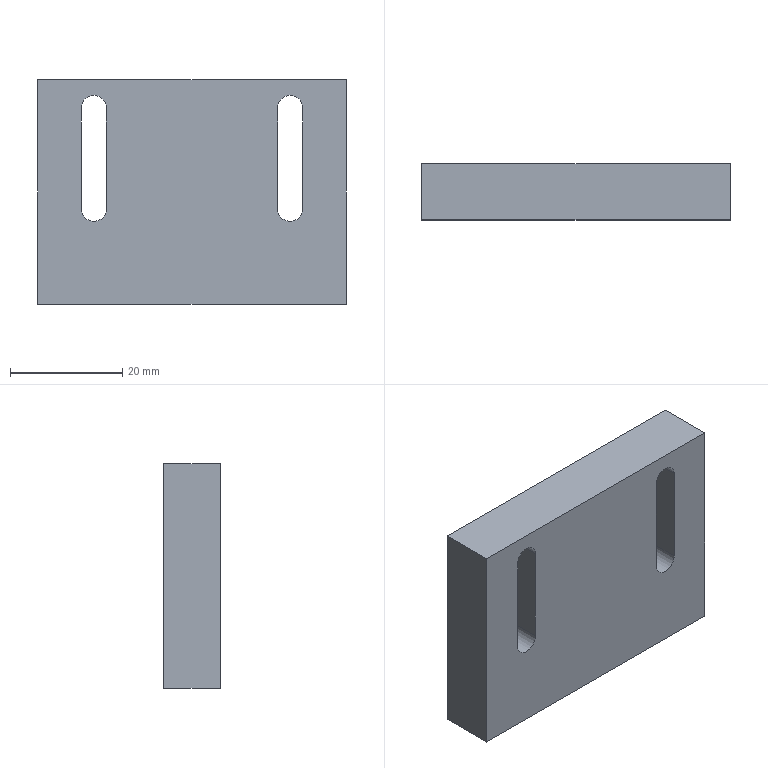Part | STEP file | PN_0007 fixture positioning -V-shape edge 1-2_Default | 1 solid | 16 faces | box 55 x 10 x 40 mm | volume 20062 mm3 | plane 10 | cylinder 6 | commonest cylinder face diameters 4.5 x6
STEP:
#1=CARTESIAN_POINT('',(0.,0.,0.));
#2=DIRECTION('',(0.,0.,1.));
#3=DIRECTION('',(1.,0.,0.));
#4=AXIS2_PLACEMENT_3D('',#1,#2,#3);
#5=CARTESIAN_POINT('',(19.75,0.,15.));
#6=VERTEX_POINT('',#5);
#7=CARTESIAN_POINT('',(19.75,10.,15.));
#8=VERTEX_POINT('',#7);
#9=CARTESIAN_POINT('',(19.75,-2.5,15.));
#10=DIRECTION('',(0.,1.,0.));
#11=VECTOR('',#10,1.);
#12=LINE('',#9,#11);
#13=CARTESIAN_POINT('',(17.5,-2.5,15.));
#14=DIRECTION('',(0.,1.,0.));
#15=DIRECTION('',(0.,0.,1.));
#16=AXIS2_PLACEMENT_3D('',#13,#14,#15);
#17=CYLINDRICAL_SURFACE('',#16,2.25);
#18=CARTESIAN_POINT('',(1.571,0.));
#19=DIRECTION('',(0.,1.));
#20=VECTOR('',#19,1.);
#21=LINE('',#18,#20);
#22=(GEOMETRIC_REPRESENTATION_CONTEXT(2)PARAMETRIC_REPRESENTATION_CONTEXT()REPRESENTATION_CONTEXT('',''));
#23=DEFINITIONAL_REPRESENTATION('',(#21),#22);
#24=PCURVE('',#17,#23);
#25=CARTESIAN_POINT('',(19.75,-2.5,-3.));
#26=DIRECTION('',(1.,0.,0.));
#27=DIRECTION('',(0.,0.,-1.));
#28=AXIS2_PLACEMENT_3D('',#25,#26,#27);
#29=PLANE('',#28);
#30=CARTESIAN_POINT('',(-18.,0.));
#31=DIRECTION('',(0.,1.));
#32=VECTOR('',#31,1.);
#33=LINE('',#30,#32);
#34=(GEOMETRIC_REPRESENTATION_CONTEXT(2)PARAMETRIC_REPRESENTATION_CONTEXT()REPRESENTATION_CONTEXT('',''));
#35=DEFINITIONAL_REPRESENTATION('',(#33),#34);
#36=PCURVE('',#29,#35);
#37=SURFACE_CURVE('',#12,(#24,#36),.PCURVE_S1.);
#38=EDGE_CURVE('',#6,#8,#37,.T.);
#39=ORIENTED_EDGE('',*,*,#38,.T.);
#40=CARTESIAN_POINT('',(17.5,10.,17.25));
#41=VERTEX_POINT('',#40);
#42=CARTESIAN_POINT('',(17.5,10.,15.));
#43=DIRECTION('',(0.,1.,0.));
#44=DIRECTION('',(0.,0.,1.));
#45=AXIS2_PLACEMENT_3D('',#42,#43,#44);
#46=CIRCLE('',#45,2.25);
#47=CARTESIAN_POINT('',(0.,12.5));
#48=DIRECTION('',(1.,0.));
#49=VECTOR('',#48,1.);
#50=LINE('',#47,#49);
#51=(GEOMETRIC_REPRESENTATION_CONTEXT(2)PARAMETRIC_REPRESENTATION_CONTEXT()REPRESENTATION_CONTEXT('',''));
#52=DEFINITIONAL_REPRESENTATION('',(#50),#51);
#53=PCURVE('',#17,#52);
#54=CARTESIAN_POINT('',(0.,10.,0.));
#55=DIRECTION('',(0.,1.,0.));
#56=DIRECTION('',(0.,0.,1.));
#57=AXIS2_PLACEMENT_3D('',#54,#55,#56);
#58=PLANE('',#57);
#59=CARTESIAN_POINT('',(15.,17.5));
#60=DIRECTION('',(1.,0.));
#61=AXIS2_PLACEMENT_2D('',#59,#60);
#62=CIRCLE('',#61,2.25);
#63=(GEOMETRIC_REPRESENTATION_CONTEXT(2)PARAMETRIC_REPRESENTATION_CONTEXT()REPRESENTATION_CONTEXT('',''));
#64=DEFINITIONAL_REPRESENTATION('',(#62),#63);
#65=PCURVE('',#58,#64);
#66=SURFACE_CURVE('',#46,(#53,#65),.PCURVE_S1.);
#67=EDGE_CURVE('',#41,#8,#66,.T.);
#68=ORIENTED_EDGE('',*,*,#67,.F.);
#69=CARTESIAN_POINT('',(17.5,0.,17.25));
#70=VERTEX_POINT('',#69);
#71=CARTESIAN_POINT('',(17.5,-2.5,17.25));
#72=DIRECTION('',(0.,1.,0.));
#73=VECTOR('',#72,1.);
#74=LINE('',#71,#73);
#75=CARTESIAN_POINT('',(0.,0.));
#76=DIRECTION('',(0.,1.));
#77=VECTOR('',#76,1.);
#78=LINE('',#75,#77);
#79=(GEOMETRIC_REPRESENTATION_CONTEXT(2)PARAMETRIC_REPRESENTATION_CONTEXT()REPRESENTATION_CONTEXT('',''));
#80=DEFINITIONAL_REPRESENTATION('',(#78),#79);
#81=PCURVE('',#17,#80);
#82=CARTESIAN_POINT('',(17.5,-2.5,15.));
#83=DIRECTION('',(0.,1.,0.));
#84=DIRECTION('',(0.,0.,1.));
#85=AXIS2_PLACEMENT_3D('',#82,#83,#84);
#86=CYLINDRICAL_SURFACE('',#85,2.25);
#87=CARTESIAN_POINT('',(6.283,0.));
#88=DIRECTION('',(0.,1.));
#89=VECTOR('',#88,1.);
#90=LINE('',#87,#89);
#91=(GEOMETRIC_REPRESENTATION_CONTEXT(2)PARAMETRIC_REPRESENTATION_CONTEXT()REPRESENTATION_CONTEXT('',''));
#92=DEFINITIONAL_REPRESENTATION('',(#90),#91);
#93=PCURVE('',#86,#92);
#94=SURFACE_CURVE('',#74,(#81,#93),.PCURVE_S1.);
#95=EDGE_CURVE('',#70,#41,#94,.T.);
#96=ORIENTED_EDGE('',*,*,#95,.F.);
#97=CARTESIAN_POINT('',(17.5,0.,15.));
#98=DIRECTION('',(0.,1.,0.));
#99=DIRECTION('',(0.,0.,1.));
#100=AXIS2_PLACEMENT_3D('',#97,#98,#99);
#101=CIRCLE('',#100,2.25);
#102=CARTESIAN_POINT('',(0.,2.5));
#103=DIRECTION('',(1.,0.));
#104=VECTOR('',#103,1.);
#105=LINE('',#102,#104);
#106=(GEOMETRIC_REPRESENTATION_CONTEXT(2)PARAMETRIC_REPRESENTATION_CONTEXT()REPRESENTATION_CONTEXT('',''));
#107=DEFINITIONAL_REPRESENTATION('',(#105),#106);
#108=PCURVE('',#17,#107);
#109=CARTESIAN_POINT('',(0.,0.,0.));
#110=DIRECTION('',(0.,1.,0.));
#111=DIRECTION('',(0.,0.,1.));
#112=AXIS2_PLACEMENT_3D('',#109,#110,#111);
#113=PLANE('',#112);
#114=CARTESIAN_POINT('',(15.,17.5));
#115=DIRECTION('',(1.,0.));
#116=AXIS2_PLACEMENT_2D('',#114,#115);
#117=CIRCLE('',#116,2.25);
#118=(GEOMETRIC_REPRESENTATION_CONTEXT(2)PARAMETRIC_REPRESENTATION_CONTEXT()REPRESENTATION_CONTEXT('',''));
#119=DEFINITIONAL_REPRESENTATION('',(#117),#118);
#120=PCURVE('',#113,#119);
#121=SURFACE_CURVE('',#101,(#108,#120),.PCURVE_S1.);
#122=EDGE_CURVE('',#70,#6,#121,.T.);
#123=ORIENTED_EDGE('',*,*,#122,.T.);
#124=EDGE_LOOP('',(#39,#68,#96,#123));
#125=FACE_BOUND('',#124,.F.);
#126=ADVANCED_FACE('',(#125),#17,.F.);
#127=CARTESIAN_POINT('',(-15.25,0.,15.));
#128=VERTEX_POINT('',#127);
#129=CARTESIAN_POINT('',(-15.25,10.,15.));
#130=VERTEX_POINT('',#129);
#131=CARTESIAN_POINT('',(-15.25,-2.5,15.));
#132=DIRECTION('',(0.,1.,0.));
#133=VECTOR('',#132,1.);
#134=LINE('',#131,#133);
#135=CARTESIAN_POINT('',(-17.5,-2.5,15.));
#136=DIRECTION('',(0.,1.,0.));
#137=DIRECTION('',(0.,0.,1.));
#138=AXIS2_PLACEMENT_3D('',#135,#136,#137);
#139=CYLINDRICAL_SURFACE('',#138,2.25);
#140=CARTESIAN_POINT('',(1.571,0.));
#141=DIRECTION('',(0.,1.));
#142=VECTOR('',#141,1.);
#143=LINE('',#140,#142);
#144=(GEOMETRIC_REPRESENTATION_CONTEXT(2)PARAMETRIC_REPRESENTATION_CONTEXT()REPRESENTATION_CONTEXT('',''));
#145=DEFINITIONAL_REPRESENTATION('',(#143),#144);
#146=PCURVE('',#139,#145);
#147=CARTESIAN_POINT('',(-15.25,-2.5,-3.));
#148=DIRECTION('',(1.,0.,0.));
#149=DIRECTION('',(0.,0.,-1.));
#150=AXIS2_PLACEMENT_3D('',#147,#148,#149);
#151=PLANE('',#150);
#152=CARTESIAN_POINT('',(-18.,0.));
#153=DIRECTION('',(0.,1.));
#154=VECTOR('',#153,1.);
#155=LINE('',#152,#154);
#156=(GEOMETRIC_REPRESENTATION_CONTEXT(2)PARAMETRIC_REPRESENTATION_CONTEXT()REPRESENTATION_CONTEXT('',''));
#157=DEFINITIONAL_REPRESENTATION('',(#155),#156);
#158=PCURVE('',#151,#157);
#159=SURFACE_CURVE('',#134,(#146,#158),.PCURVE_S1.);
#160=EDGE_CURVE('',#128,#130,#159,.T.);
#161=ORIENTED_EDGE('',*,*,#160,.T.);
#162=CARTESIAN_POINT('',(-17.5,10.,17.25));
#163=VERTEX_POINT('',#162);
#164=CARTESIAN_POINT('',(-17.5,10.,15.));
#165=DIRECTION('',(0.,1.,0.));
#166=DIRECTION('',(0.,0.,1.));
#167=AXIS2_PLACEMENT_3D('',#164,#165,#166);
#168=CIRCLE('',#167,2.25);
#169=CARTESIAN_POINT('',(0.,12.5));
#170=DIRECTION('',(1.,0.));
#171=VECTOR('',#170,1.);
#172=LINE('',#169,#171);
#173=(GEOMETRIC_REPRESENTATION_CONTEXT(2)PARAMETRIC_REPRESENTATION_CONTEXT()REPRESENTATION_CONTEXT('',''));
#174=DEFINITIONAL_REPRESENTATION('',(#172),#173);
#175=PCURVE('',#139,#174);
#176=CARTESIAN_POINT('',(15.,-17.5));
#177=DIRECTION('',(1.,0.));
#178=AXIS2_PLACEMENT_2D('',#176,#177);
#179=CIRCLE('',#178,2.25);
#180=(GEOMETRIC_REPRESENTATION_CONTEXT(2)PARAMETRIC_REPRESENTATION_CONTEXT()REPRESENTATION_CONTEXT('',''));
#181=DEFINITIONAL_REPRESENTATION('',(#179),#180);
#182=PCURVE('',#58,#181);
#183=SURFACE_CURVE('',#168,(#175,#182),.PCURVE_S1.);
#184=EDGE_CURVE('',#163,#130,#183,.T.);
#185=ORIENTED_EDGE('',*,*,#184,.F.);
#186=CARTESIAN_POINT('',(-17.5,0.,17.25));
#187=VERTEX_POINT('',#186);
#188=CARTESIAN_POINT('',(-17.5,-2.5,17.25));
#189=DIRECTION('',(0.,1.,0.));
#190=VECTOR('',#189,1.);
#191=LINE('',#188,#190);
#192=CARTESIAN_POINT('',(0.,0.));
#193=DIRECTION('',(0.,1.));
#194=VECTOR('',#193,1.);
#195=LINE('',#192,#194);
#196=(GEOMETRIC_REPRESENTATION_CONTEXT(2)PARAMETRIC_REPRESENTATION_CONTEXT()REPRESENTATION_CONTEXT('',''));
#197=DEFINITIONAL_REPRESENTATION('',(#195),#196);
#198=PCURVE('',#139,#197);
#199=CARTESIAN_POINT('',(-17.5,-2.5,15.));
#200=DIRECTION('',(0.,1.,0.));
#201=DIRECTION('',(0.,0.,1.));
#202=AXIS2_PLACEMENT_3D('',#199,#200,#201);
#203=CYLINDRICAL_SURFACE('',#202,2.25);
#204=CARTESIAN_POINT('',(6.283,0.));
#205=DIRECTION('',(0.,1.));
#206=VECTOR('',#205,1.);
#207=LINE('',#204,#206);
#208=(GEOMETRIC_REPRESENTATION_CONTEXT(2)PARAMETRIC_REPRESENTATION_CONTEXT()REPRESENTATION_CONTEXT('',''));
#209=DEFINITIONAL_REPRESENTATION('',(#207),#208);
#210=PCURVE('',#203,#209);
#211=SURFACE_CURVE('',#191,(#198,#210),.PCURVE_S1.);
#212=EDGE_CURVE('',#187,#163,#211,.T.);
#213=ORIENTED_EDGE('',*,*,#212,.F.);
#214=CARTESIAN_POINT('',(-17.5,0.,15.));
#215=DIRECTION('',(0.,1.,0.));
#216=DIRECTION('',(0.,0.,1.));
#217=AXIS2_PLACEMENT_3D('',#214,#215,#216);
#218=CIRCLE('',#217,2.25);
#219=CARTESIAN_POINT('',(0.,2.5));
#220=DIRECTION('',(1.,0.));
#221=VECTOR('',#220,1.);
#222=LINE('',#219,#221);
#223=(GEOMETRIC_REPRESENTATION_CONTEXT(2)PARAMETRIC_REPRESENTATION_CONTEXT()REPRESENTATION_CONTEXT('',''));
#224=DEFINITIONAL_REPRESENTATION('',(#222),#223);
#225=PCURVE('',#139,#224);
#226=CARTESIAN_POINT('',(15.,-17.5));
#227=DIRECTION('',(1.,0.));
#228=AXIS2_PLACEMENT_2D('',#226,#227);
#229=CIRCLE('',#228,2.25);
#230=(GEOMETRIC_REPRESENTATION_CONTEXT(2)PARAMETRIC_REPRESENTATION_CONTEXT()REPRESENTATION_CONTEXT('',''));
#231=DEFINITIONAL_REPRESENTATION('',(#229),#230);
#232=PCURVE('',#113,#231);
#233=SURFACE_CURVE('',#218,(#225,#232),.PCURVE_S1.);
#234=EDGE_CURVE('',#187,#128,#233,.T.);
#235=ORIENTED_EDGE('',*,*,#234,.T.);
#236=EDGE_LOOP('',(#161,#185,#213,#235));
#237=FACE_BOUND('',#236,.F.);
#238=ADVANCED_FACE('',(#237),#139,.F.);
#239=CARTESIAN_POINT('',(27.5,0.,20.));
#240=VERTEX_POINT('',#239);
#241=CARTESIAN_POINT('',(27.5,0.,-20.));
#242=VERTEX_POINT('',#241);
#243=CARTESIAN_POINT('',(27.5,0.,-20.));
#244=DIRECTION('',(0.,0.,-1.));
#245=VECTOR('',#244,1.);
#246=LINE('',#243,#245);
#247=CARTESIAN_POINT('',(27.5,10.,-20.));
#248=DIRECTION('',(-1.,0.,0.));
#249=DIRECTION('',(0.,0.,1.));
#250=AXIS2_PLACEMENT_3D('',#247,#248,#249);
#251=PLANE('',#250);
#252=CARTESIAN_POINT('',(0.,-10.));
#253=DIRECTION('',(-1.,0.));
#254=VECTOR('',#253,1.);
#255=LINE('',#252,#254);
#256=(GEOMETRIC_REPRESENTATION_CONTEXT(2)PARAMETRIC_REPRESENTATION_CONTEXT()REPRESENTATION_CONTEXT('',''));
#257=DEFINITIONAL_REPRESENTATION('',(#255),#256);
#258=PCURVE('',#251,#257);
#259=CARTESIAN_POINT('',(-20.,27.5));
#260=DIRECTION('',(-1.,0.));
#261=VECTOR('',#260,1.);
#262=LINE('',#259,#261);
#263=(GEOMETRIC_REPRESENTATION_CONTEXT(2)PARAMETRIC_REPRESENTATION_CONTEXT()REPRESENTATION_CONTEXT('',''));
#264=DEFINITIONAL_REPRESENTATION('',(#262),#263);
#265=PCURVE('',#113,#264);
#266=SURFACE_CURVE('',#246,(#258,#265),.PCURVE_S1.);
#267=EDGE_CURVE('',#240,#242,#266,.T.);
#268=ORIENTED_EDGE('',*,*,#267,.T.);
#269=CARTESIAN_POINT('',(27.5,10.,-20.));
#270=VERTEX_POINT('',#269);
#271=CARTESIAN_POINT('',(27.5,10.,-20.));
#272=DIRECTION('',(0.,-1.,0.));
#273=VECTOR('',#272,1.);
#274=LINE('',#271,#273);
#275=CARTESIAN_POINT('',(0.,0.));
#276=DIRECTION('',(0.,-1.));
#277=VECTOR('',#276,1.);
#278=LINE('',#275,#277);
#279=(GEOMETRIC_REPRESENTATION_CONTEXT(2)PARAMETRIC_REPRESENTATION_CONTEXT()REPRESENTATION_CONTEXT('',''));
#280=DEFINITIONAL_REPRESENTATION('',(#278),#279);
#281=PCURVE('',#251,#280);
#282=CARTESIAN_POINT('',(-27.5,10.,-20.));
#283=DIRECTION('',(0.,0.,1.));
#284=DIRECTION('',(1.,0.,0.));
#285=AXIS2_PLACEMENT_3D('',#282,#283,#284);
#286=PLANE('',#285);
#287=CARTESIAN_POINT('',(55.,0.));
#288=DIRECTION('',(0.,-1.));
#289=VECTOR('',#288,1.);
#290=LINE('',#287,#289);
#291=(GEOMETRIC_REPRESENTATION_CONTEXT(2)PARAMETRIC_REPRESENTATION_CONTEXT()REPRESENTATION_CONTEXT('',''));
#292=DEFINITIONAL_REPRESENTATION('',(#290),#291);
#293=PCURVE('',#286,#292);
#294=SURFACE_CURVE('',#274,(#281,#293),.PCURVE_S1.);
#295=EDGE_CURVE('',#270,#242,#294,.T.);
#296=ORIENTED_EDGE('',*,*,#295,.F.);
#297=CARTESIAN_POINT('',(27.5,10.,20.));
#298=VERTEX_POINT('',#297);
#299=CARTESIAN_POINT('',(27.5,10.,-20.));
#300=DIRECTION('',(0.,0.,-1.));
#301=VECTOR('',#300,1.);
#302=LINE('',#299,#301);
#303=CARTESIAN_POINT('',(0.,0.));
#304=DIRECTION('',(-1.,0.));
#305=VECTOR('',#304,1.);
#306=LINE('',#303,#305);
#307=(GEOMETRIC_REPRESENTATION_CONTEXT(2)PARAMETRIC_REPRESENTATION_CONTEXT()REPRESENTATION_CONTEXT('',''));
#308=DEFINITIONAL_REPRESENTATION('',(#306),#307);
#309=PCURVE('',#251,#308);
#310=CARTESIAN_POINT('',(-20.,27.5));
#311=DIRECTION('',(-1.,0.));
#312=VECTOR('',#311,1.);
#313=LINE('',#310,#312);
#314=(GEOMETRIC_REPRESENTATION_CONTEXT(2)PARAMETRIC_REPRESENTATION_CONTEXT()REPRESENTATION_CONTEXT('',''));
#315=DEFINITIONAL_REPRESENTATION('',(#313),#314);
#316=PCURVE('',#58,#315);
#317=SURFACE_CURVE('',#302,(#309,#316),.PCURVE_S1.);
#318=EDGE_CURVE('',#298,#270,#317,.T.);
#319=ORIENTED_EDGE('',*,*,#318,.F.);
#320=CARTESIAN_POINT('',(27.5,10.,20.));
#321=DIRECTION('',(0.,-1.,0.));
#322=VECTOR('',#321,1.);
#323=LINE('',#320,#322);
#324=CARTESIAN_POINT('',(40.,0.));
#325=DIRECTION('',(0.,-1.));
#326=VECTOR('',#325,1.);
#327=LINE('',#324,#326);
#328=(GEOMETRIC_REPRESENTATION_CONTEXT(2)PARAMETRIC_REPRESENTATION_CONTEXT()REPRESENTATION_CONTEXT('',''));
#329=DEFINITIONAL_REPRESENTATION('',(#327),#328);
#330=PCURVE('',#251,#329);
#331=CARTESIAN_POINT('',(-27.5,10.,20.));
#332=DIRECTION('',(0.,0.,-1.));
#333=DIRECTION('',(-1.,0.,0.));
#334=AXIS2_PLACEMENT_3D('',#331,#332,#333);
#335=PLANE('',#334);
#336=CARTESIAN_POINT('',(-55.,0.));
#337=DIRECTION('',(0.,-1.));
#338=VECTOR('',#337,1.);
#339=LINE('',#336,#338);
#340=(GEOMETRIC_REPRESENTATION_CONTEXT(2)PARAMETRIC_REPRESENTATION_CONTEXT()REPRESENTATION_CONTEXT('',''));
#341=DEFINITIONAL_REPRESENTATION('',(#339),#340);
#342=PCURVE('',#335,#341);
#343=SURFACE_CURVE('',#323,(#330,#342),.PCURVE_S1.);
#344=EDGE_CURVE('',#298,#240,#343,.T.);
#345=ORIENTED_EDGE('',*,*,#344,.T.);
#346=EDGE_LOOP('',(#268,#296,#319,#345));
#347=FACE_BOUND('',#346,.T.);
#348=ADVANCED_FACE('',(#347),#251,.F.);
#349=CARTESIAN_POINT('',(-27.5,0.,-20.));
#350=VERTEX_POINT('',#349);
#351=CARTESIAN_POINT('',(-27.5,0.,-20.));
#352=DIRECTION('',(-1.,0.,0.));
#353=VECTOR('',#352,1.);
#354=LINE('',#351,#353);
#355=CARTESIAN_POINT('',(0.,-10.));
#356=DIRECTION('',(-1.,0.));
#357=VECTOR('',#356,1.);
#358=LINE('',#355,#357);
#359=(GEOMETRIC_REPRESENTATION_CONTEXT(2)PARAMETRIC_REPRESENTATION_CONTEXT()REPRESENTATION_CONTEXT('',''));
#360=DEFINITIONAL_REPRESENTATION('',(#358),#359);
#361=PCURVE('',#286,#360);
#362=CARTESIAN_POINT('',(-20.,-27.5));
#363=DIRECTION('',(0.,-1.));
#364=VECTOR('',#363,1.);
#365=LINE('',#362,#364);
#366=(GEOMETRIC_REPRESENTATION_CONTEXT(2)PARAMETRIC_REPRESENTATION_CONTEXT()REPRESENTATION_CONTEXT('',''));
#367=DEFINITIONAL_REPRESENTATION('',(#365),#366);
#368=PCURVE('',#113,#367);
#369=SURFACE_CURVE('',#354,(#361,#368),.PCURVE_S1.);
#370=EDGE_CURVE('',#242,#350,#369,.T.);
#371=ORIENTED_EDGE('',*,*,#370,.T.);
#372=CARTESIAN_POINT('',(-27.5,10.,-20.));
#373=VERTEX_POINT('',#372);
#374=CARTESIAN_POINT('',(-27.5,10.,-20.));
#375=DIRECTION('',(0.,-1.,0.));
#376=VECTOR('',#375,1.);
#377=LINE('',#374,#376);
#378=CARTESIAN_POINT('',(0.,0.));
#379=DIRECTION('',(0.,-1.));
#380=VECTOR('',#379,1.);
#381=LINE('',#378,#380);
#382=(GEOMETRIC_REPRESENTATION_CONTEXT(2)PARAMETRIC_REPRESENTATION_CONTEXT()REPRESENTATION_CONTEXT('',''));
#383=DEFINITIONAL_REPRESENTATION('',(#381),#382);
#384=PCURVE('',#286,#383);
#385=CARTESIAN_POINT('',(-27.5,10.,-20.));
#386=DIRECTION('',(1.,0.,0.));
#387=DIRECTION('',(0.,0.,-1.));
#388=AXIS2_PLACEMENT_3D('',#385,#386,#387);
#389=PLANE('',#388);
#390=CARTESIAN_POINT('',(0.,0.));
#391=DIRECTION('',(0.,-1.));
#392=VECTOR('',#391,1.);
#393=LINE('',#390,#392);
#394=(GEOMETRIC_REPRESENTATION_CONTEXT(2)PARAMETRIC_REPRESENTATION_CONTEXT()REPRESENTATION_CONTEXT('',''));
#395=DEFINITIONAL_REPRESENTATION('',(#393),#394);
#396=PCURVE('',#389,#395);
#397=SURFACE_CURVE('',#377,(#384,#396),.PCURVE_S1.);
#398=EDGE_CURVE('',#373,#350,#397,.T.);
#399=ORIENTED_EDGE('',*,*,#398,.F.);
#400=CARTESIAN_POINT('',(-27.5,10.,-20.));
#401=DIRECTION('',(-1.,0.,0.));
#402=VECTOR('',#401,1.);
#403=LINE('',#400,#402);
#404=CARTESIAN_POINT('',(0.,0.));
#405=DIRECTION('',(-1.,0.));
#406=VECTOR('',#405,1.);
#407=LINE('',#404,#406);
#408=(GEOMETRIC_REPRESENTATION_CONTEXT(2)PARAMETRIC_REPRESENTATION_CONTEXT()REPRESENTATION_CONTEXT('',''));
#409=DEFINITIONAL_REPRESENTATION('',(#407),#408);
#410=PCURVE('',#286,#409);
#411=CARTESIAN_POINT('',(-20.,-27.5));
#412=DIRECTION('',(0.,-1.));
#413=VECTOR('',#412,1.);
#414=LINE('',#411,#413);
#415=(GEOMETRIC_REPRESENTATION_CONTEXT(2)PARAMETRIC_REPRESENTATION_CONTEXT()REPRESENTATION_CONTEXT('',''));
#416=DEFINITIONAL_REPRESENTATION('',(#414),#415);
#417=PCURVE('',#58,#416);
#418=SURFACE_CURVE('',#403,(#410,#417),.PCURVE_S1.);
#419=EDGE_CURVE('',#270,#373,#418,.T.);
#420=ORIENTED_EDGE('',*,*,#419,.F.);
#421=ORIENTED_EDGE('',*,*,#295,.T.);
#422=EDGE_LOOP('',(#371,#399,#420,#421));
#423=FACE_BOUND('',#422,.T.);
#424=ADVANCED_FACE('',(#423),#286,.F.);
#425=CARTESIAN_POINT('',(-27.5,0.,20.));
#426=VERTEX_POINT('',#425);
#427=CARTESIAN_POINT('',(-27.5,0.,-20.));
#428=DIRECTION('',(0.,0.,1.));
#429=VECTOR('',#428,1.);
#430=LINE('',#427,#429);
#431=CARTESIAN_POINT('',(0.,-10.));
#432=DIRECTION('',(-1.,0.));
#433=VECTOR('',#432,1.);
#434=LINE('',#431,#433);
#435=(GEOMETRIC_REPRESENTATION_CONTEXT(2)PARAMETRIC_REPRESENTATION_CONTEXT()REPRESENTATION_CONTEXT('',''));
#436=DEFINITIONAL_REPRESENTATION('',(#434),#435);
#437=PCURVE('',#389,#436);
#438=CARTESIAN_POINT('',(-20.,-27.5));
#439=DIRECTION('',(1.,0.));
#440=VECTOR('',#439,1.);
#441=LINE('',#438,#440);
#442=(GEOMETRIC_REPRESENTATION_CONTEXT(2)PARAMETRIC_REPRESENTATION_CONTEXT()REPRESENTATION_CONTEXT('',''));
#443=DEFINITIONAL_REPRESENTATION('',(#441),#442);
#444=PCURVE('',#113,#443);
#445=SURFACE_CURVE('',#430,(#437,#444),.PCURVE_S1.);
#446=EDGE_CURVE('',#350,#426,#445,.T.);
#447=ORIENTED_EDGE('',*,*,#446,.T.);
#448=CARTESIAN_POINT('',(-27.5,10.,20.));
#449=VERTEX_POINT('',#448);
#450=CARTESIAN_POINT('',(-27.5,10.,20.));
#451=DIRECTION('',(0.,-1.,0.));
#452=VECTOR('',#451,1.);
#453=LINE('',#450,#452);
#454=CARTESIAN_POINT('',(-40.,0.));
#455=DIRECTION('',(0.,-1.));
#456=VECTOR('',#455,1.);
#457=LINE('',#454,#456);
#458=(GEOMETRIC_REPRESENTATION_CONTEXT(2)PARAMETRIC_REPRESENTATION_CONTEXT()REPRESENTATION_CONTEXT('',''));
#459=DEFINITIONAL_REPRESENTATION('',(#457),#458);
#460=PCURVE('',#389,#459);
#461=CARTESIAN_POINT('',(0.,0.));
#462=DIRECTION('',(0.,-1.));
#463=VECTOR('',#462,1.);
#464=LINE('',#461,#463);
#465=(GEOMETRIC_REPRESENTATION_CONTEXT(2)PARAMETRIC_REPRESENTATION_CONTEXT()REPRESENTATION_CONTEXT('',''));
#466=DEFINITIONAL_REPRESENTATION('',(#464),#465);
#467=PCURVE('',#335,#466);
#468=SURFACE_CURVE('',#453,(#460,#467),.PCURVE_S1.);
#469=EDGE_CURVE('',#449,#426,#468,.T.);
#470=ORIENTED_EDGE('',*,*,#469,.F.);
#471=CARTESIAN_POINT('',(-27.5,10.,-20.));
#472=DIRECTION('',(0.,0.,1.));
#473=VECTOR('',#472,1.);
#474=LINE('',#471,#473);
#475=CARTESIAN_POINT('',(0.,0.));
#476=DIRECTION('',(-1.,0.));
#477=VECTOR('',#476,1.);
#478=LINE('',#475,#477);
#479=(GEOMETRIC_REPRESENTATION_CONTEXT(2)PARAMETRIC_REPRESENTATION_CONTEXT()REPRESENTATION_CONTEXT('',''));
#480=DEFINITIONAL_REPRESENTATION('',(#478),#479);
#481=PCURVE('',#389,#480);
#482=CARTESIAN_POINT('',(-20.,-27.5));
#483=DIRECTION('',(1.,0.));
#484=VECTOR('',#483,1.);
#485=LINE('',#482,#484);
#486=(GEOMETRIC_REPRESENTATION_CONTEXT(2)PARAMETRIC_REPRESENTATION_CONTEXT()REPRESENTATION_CONTEXT('',''));
#487=DEFINITIONAL_REPRESENTATION('',(#485),#486);
#488=PCURVE('',#58,#487);
#489=SURFACE_CURVE('',#474,(#481,#488),.PCURVE_S1.);
#490=EDGE_CURVE('',#373,#449,#489,.T.);
#491=ORIENTED_EDGE('',*,*,#490,.F.);
#492=ORIENTED_EDGE('',*,*,#398,.T.);
#493=EDGE_LOOP('',(#447,#470,#491,#492));
#494=FACE_BOUND('',#493,.T.);
#495=ADVANCED_FACE('',(#494),#389,.F.);
#496=CARTESIAN_POINT('',(-27.5,0.,20.));
#497=DIRECTION('',(1.,0.,0.));
#498=VECTOR('',#497,1.);
#499=LINE('',#496,#498);
#500=CARTESIAN_POINT('',(0.,-10.));
#501=DIRECTION('',(-1.,0.));
#502=VECTOR('',#501,1.);
#503=LINE('',#500,#502);
#504=(GEOMETRIC_REPRESENTATION_CONTEXT(2)PARAMETRIC_REPRESENTATION_CONTEXT()REPRESENTATION_CONTEXT('',''));
#505=DEFINITIONAL_REPRESENTATION('',(#503),#504);
#506=PCURVE('',#335,#505);
#507=CARTESIAN_POINT('',(20.,-27.5));
#508=DIRECTION('',(0.,1.));
#509=VECTOR('',#508,1.);
#510=LINE('',#507,#509);
#511=(GEOMETRIC_REPRESENTATION_CONTEXT(2)PARAMETRIC_REPRESENTATION_CONTEXT()REPRESENTATION_CONTEXT('',''));
#512=DEFINITIONAL_REPRESENTATION('',(#510),#511);
#513=PCURVE('',#113,#512);
#514=SURFACE_CURVE('',#499,(#506,#513),.PCURVE_S1.);
#515=EDGE_CURVE('',#426,#240,#514,.T.);
#516=ORIENTED_EDGE('',*,*,#515,.T.);
#517=ORIENTED_EDGE('',*,*,#344,.F.);
#518=CARTESIAN_POINT('',(-27.5,10.,20.));
#519=DIRECTION('',(1.,0.,0.));
#520=VECTOR('',#519,1.);
#521=LINE('',#518,#520);
#522=CARTESIAN_POINT('',(0.,0.));
#523=DIRECTION('',(-1.,0.));
#524=VECTOR('',#523,1.);
#525=LINE('',#522,#524);
#526=(GEOMETRIC_REPRESENTATION_CONTEXT(2)PARAMETRIC_REPRESENTATION_CONTEXT()REPRESENTATION_CONTEXT('',''));
#527=DEFINITIONAL_REPRESENTATION('',(#525),#526);
#528=PCURVE('',#335,#527);
#529=CARTESIAN_POINT('',(20.,-27.5));
#530=DIRECTION('',(0.,1.));
#531=VECTOR('',#530,1.);
#532=LINE('',#529,#531);
#533=(GEOMETRIC_REPRESENTATION_CONTEXT(2)PARAMETRIC_REPRESENTATION_CONTEXT()REPRESENTATION_CONTEXT('',''));
#534=DEFINITIONAL_REPRESENTATION('',(#532),#533);
#535=PCURVE('',#58,#534);
#536=SURFACE_CURVE('',#521,(#528,#535),.PCURVE_S1.);
#537=EDGE_CURVE('',#449,#298,#536,.T.);
#538=ORIENTED_EDGE('',*,*,#537,.F.);
#539=ORIENTED_EDGE('',*,*,#469,.T.);
#540=EDGE_LOOP('',(#516,#517,#538,#539));
#541=FACE_BOUND('',#540,.T.);
#542=ADVANCED_FACE('',(#541),#335,.F.);
#543=CARTESIAN_POINT('',(19.75,10.,-3.));
#544=VERTEX_POINT('',#543);
#545=CARTESIAN_POINT('',(15.25,10.,-3.));
#546=VERTEX_POINT('',#545);
#547=CARTESIAN_POINT('',(17.5,10.,-3.));
#548=DIRECTION('',(0.,1.,0.));
#549=DIRECTION('',(0.,0.,1.));
#550=AXIS2_PLACEMENT_3D('',#547,#548,#549);
#551=CIRCLE('',#550,2.25);
#552=CARTESIAN_POINT('',(-3.,17.5));
#553=DIRECTION('',(1.,0.));
#554=AXIS2_PLACEMENT_2D('',#552,#553);
#555=CIRCLE('',#554,2.25);
#556=(GEOMETRIC_REPRESENTATION_CONTEXT(2)PARAMETRIC_REPRESENTATION_CONTEXT()REPRESENTATION_CONTEXT('',''));
#557=DEFINITIONAL_REPRESENTATION('',(#555),#556);
#558=PCURVE('',#58,#557);
#559=CARTESIAN_POINT('',(17.5,-2.5,-3.));
#560=DIRECTION('',(0.,1.,0.));
#561=DIRECTION('',(0.,0.,1.));
#562=AXIS2_PLACEMENT_3D('',#559,#560,#561);
#563=CYLINDRICAL_SURFACE('',#562,2.25);
#564=CARTESIAN_POINT('',(0.,12.5));
#565=DIRECTION('',(1.,0.));
#566=VECTOR('',#565,1.);
#567=LINE('',#564,#566);
#568=(GEOMETRIC_REPRESENTATION_CONTEXT(2)PARAMETRIC_REPRESENTATION_CONTEXT()REPRESENTATION_CONTEXT('',''));
#569=DEFINITIONAL_REPRESENTATION('',(#567),#568);
#570=PCURVE('',#563,#569);
#571=SURFACE_CURVE('',#551,(#558,#570),.PCURVE_S1.);
#572=EDGE_CURVE('',#544,#546,#571,.T.);
#573=ORIENTED_EDGE('',*,*,#572,.F.);
#574=CARTESIAN_POINT('',(19.75,10.,-3.));
#575=DIRECTION('',(0.,0.,-1.));
#576=VECTOR('',#575,1.);
#577=LINE('',#574,#576);
#578=CARTESIAN_POINT('',(-3.,19.75));
#579=DIRECTION('',(-1.,0.));
#580=VECTOR('',#579,1.);
#581=LINE('',#578,#580);
#582=(GEOMETRIC_REPRESENTATION_CONTEXT(2)PARAMETRIC_REPRESENTATION_CONTEXT()REPRESENTATION_CONTEXT('',''));
#583=DEFINITIONAL_REPRESENTATION('',(#581),#582);
#584=PCURVE('',#58,#583);
#585=CARTESIAN_POINT('',(0.,12.5));
#586=DIRECTION('',(1.,0.));
#587=VECTOR('',#586,1.);
#588=LINE('',#585,#587);
#589=(GEOMETRIC_REPRESENTATION_CONTEXT(2)PARAMETRIC_REPRESENTATION_CONTEXT()REPRESENTATION_CONTEXT('',''));
#590=DEFINITIONAL_REPRESENTATION('',(#588),#589);
#591=PCURVE('',#29,#590);
#592=SURFACE_CURVE('',#577,(#584,#591),.PCURVE_S1.);
#593=EDGE_CURVE('',#8,#544,#592,.T.);
#594=ORIENTED_EDGE('',*,*,#593,.F.);
#595=ORIENTED_EDGE('',*,*,#67,.F.);
#596=CARTESIAN_POINT('',(15.25,10.,15.));
#597=VERTEX_POINT('',#596);
#598=CARTESIAN_POINT('',(17.5,10.,15.));
#599=DIRECTION('',(0.,1.,0.));
#600=DIRECTION('',(0.,0.,1.));
#601=AXIS2_PLACEMENT_3D('',#598,#599,#600);
#602=CIRCLE('',#601,2.25);
#603=CARTESIAN_POINT('',(15.,17.5));
#604=DIRECTION('',(1.,0.));
#605=AXIS2_PLACEMENT_2D('',#603,#604);
#606=CIRCLE('',#605,2.25);
#607=(GEOMETRIC_REPRESENTATION_CONTEXT(2)PARAMETRIC_REPRESENTATION_CONTEXT()REPRESENTATION_CONTEXT('',''));
#608=DEFINITIONAL_REPRESENTATION('',(#606),#607);
#609=PCURVE('',#58,#608);
#610=CARTESIAN_POINT('',(0.,12.5));
#611=DIRECTION('',(1.,0.));
#612=VECTOR('',#611,1.);
#613=LINE('',#610,#612);
#614=(GEOMETRIC_REPRESENTATION_CONTEXT(2)PARAMETRIC_REPRESENTATION_CONTEXT()REPRESENTATION_CONTEXT('',''));
#615=DEFINITIONAL_REPRESENTATION('',(#613),#614);
#616=PCURVE('',#86,#615);
#617=SURFACE_CURVE('',#602,(#609,#616),.PCURVE_S1.);
#618=EDGE_CURVE('',#597,#41,#617,.T.);
#619=ORIENTED_EDGE('',*,*,#618,.F.);
#620=CARTESIAN_POINT('',(15.25,10.,-3.));
#621=DIRECTION('',(0.,0.,1.));
#622=VECTOR('',#621,1.);
#623=LINE('',#620,#622);
#624=CARTESIAN_POINT('',(-3.,15.25));
#625=DIRECTION('',(1.,0.));
#626=VECTOR('',#625,1.);
#627=LINE('',#624,#626);
#628=(GEOMETRIC_REPRESENTATION_CONTEXT(2)PARAMETRIC_REPRESENTATION_CONTEXT()REPRESENTATION_CONTEXT('',''));
#629=DEFINITIONAL_REPRESENTATION('',(#627),#628);
#630=PCURVE('',#58,#629);
#631=CARTESIAN_POINT('',(15.25,-2.5,-3.));
#632=DIRECTION('',(-1.,0.,0.));
#633=DIRECTION('',(0.,0.,1.));
#634=AXIS2_PLACEMENT_3D('',#631,#632,#633);
#635=PLANE('',#634);
#636=CARTESIAN_POINT('',(0.,12.5));
#637=DIRECTION('',(1.,0.));
#638=VECTOR('',#637,1.);
#639=LINE('',#636,#638);
#640=(GEOMETRIC_REPRESENTATION_CONTEXT(2)PARAMETRIC_REPRESENTATION_CONTEXT()REPRESENTATION_CONTEXT('',''));
#641=DEFINITIONAL_REPRESENTATION('',(#639),#640);
#642=PCURVE('',#635,#641);
#643=SURFACE_CURVE('',#623,(#630,#642),.PCURVE_S1.);
#644=EDGE_CURVE('',#546,#597,#643,.T.);
#645=ORIENTED_EDGE('',*,*,#644,.F.);
#646=EDGE_LOOP('',(#573,#594,#595,#619,#645));
#647=FACE_BOUND('',#646,.T.);
#648=CARTESIAN_POINT('',(-15.25,10.,-3.));
#649=VERTEX_POINT('',#648);
#650=CARTESIAN_POINT('',(-19.75,10.,-3.));
#651=VERTEX_POINT('',#650);
#652=CARTESIAN_POINT('',(-17.5,10.,-3.));
#653=DIRECTION('',(0.,1.,0.));
#654=DIRECTION('',(0.,0.,1.));
#655=AXIS2_PLACEMENT_3D('',#652,#653,#654);
#656=CIRCLE('',#655,2.25);
#657=CARTESIAN_POINT('',(-3.,-17.5));
#658=DIRECTION('',(1.,0.));
#659=AXIS2_PLACEMENT_2D('',#657,#658);
#660=CIRCLE('',#659,2.25);
#661=(GEOMETRIC_REPRESENTATION_CONTEXT(2)PARAMETRIC_REPRESENTATION_CONTEXT()REPRESENTATION_CONTEXT('',''));
#662=DEFINITIONAL_REPRESENTATION('',(#660),#661);
#663=PCURVE('',#58,#662);
#664=CARTESIAN_POINT('',(-17.5,-2.5,-3.));
#665=DIRECTION('',(0.,1.,0.));
#666=DIRECTION('',(0.,0.,1.));
#667=AXIS2_PLACEMENT_3D('',#664,#665,#666);
#668=CYLINDRICAL_SURFACE('',#667,2.25);
#669=CARTESIAN_POINT('',(0.,12.5));
#670=DIRECTION('',(1.,0.));
#671=VECTOR('',#670,1.);
#672=LINE('',#669,#671);
#673=(GEOMETRIC_REPRESENTATION_CONTEXT(2)PARAMETRIC_REPRESENTATION_CONTEXT()REPRESENTATION_CONTEXT('',''));
#674=DEFINITIONAL_REPRESENTATION('',(#672),#673);
#675=PCURVE('',#668,#674);
#676=SURFACE_CURVE('',#656,(#663,#675),.PCURVE_S1.);
#677=EDGE_CURVE('',#649,#651,#676,.T.);
#678=ORIENTED_EDGE('',*,*,#677,.F.);
#679=CARTESIAN_POINT('',(-15.25,10.,-3.));
#680=DIRECTION('',(0.,0.,-1.));
#681=VECTOR('',#680,1.);
#682=LINE('',#679,#681);
#683=CARTESIAN_POINT('',(-3.,-15.25));
#684=DIRECTION('',(-1.,0.));
#685=VECTOR('',#684,1.);
#686=LINE('',#683,#685);
#687=(GEOMETRIC_REPRESENTATION_CONTEXT(2)PARAMETRIC_REPRESENTATION_CONTEXT()REPRESENTATION_CONTEXT('',''));
#688=DEFINITIONAL_REPRESENTATION('',(#686),#687);
#689=PCURVE('',#58,#688);
#690=CARTESIAN_POINT('',(0.,12.5));
#691=DIRECTION('',(1.,0.));
#692=VECTOR('',#691,1.);
#693=LINE('',#690,#692);
#694=(GEOMETRIC_REPRESENTATION_CONTEXT(2)PARAMETRIC_REPRESENTATION_CONTEXT()REPRESENTATION_CONTEXT('',''));
#695=DEFINITIONAL_REPRESENTATION('',(#693),#694);
#696=PCURVE('',#151,#695);
#697=SURFACE_CURVE('',#682,(#689,#696),.PCURVE_S1.);
#698=EDGE_CURVE('',#130,#649,#697,.T.);
#699=ORIENTED_EDGE('',*,*,#698,.F.);
#700=ORIENTED_EDGE('',*,*,#184,.F.);
#701=CARTESIAN_POINT('',(-19.75,10.,15.));
#702=VERTEX_POINT('',#701);
#703=CARTESIAN_POINT('',(-17.5,10.,15.));
#704=DIRECTION('',(0.,1.,0.));
#705=DIRECTION('',(0.,0.,1.));
#706=AXIS2_PLACEMENT_3D('',#703,#704,#705);
#707=CIRCLE('',#706,2.25);
#708=CARTESIAN_POINT('',(15.,-17.5));
#709=DIRECTION('',(1.,0.));
#710=AXIS2_PLACEMENT_2D('',#708,#709);
#711=CIRCLE('',#710,2.25);
#712=(GEOMETRIC_REPRESENTATION_CONTEXT(2)PARAMETRIC_REPRESENTATION_CONTEXT()REPRESENTATION_CONTEXT('',''));
#713=DEFINITIONAL_REPRESENTATION('',(#711),#712);
#714=PCURVE('',#58,#713);
#715=CARTESIAN_POINT('',(0.,12.5));
#716=DIRECTION('',(1.,0.));
#717=VECTOR('',#716,1.);
#718=LINE('',#715,#717);
#719=(GEOMETRIC_REPRESENTATION_CONTEXT(2)PARAMETRIC_REPRESENTATION_CONTEXT()REPRESENTATION_CONTEXT('',''));
#720=DEFINITIONAL_REPRESENTATION('',(#718),#719);
#721=PCURVE('',#203,#720);
#722=SURFACE_CURVE('',#707,(#714,#721),.PCURVE_S1.);
#723=EDGE_CURVE('',#702,#163,#722,.T.);
#724=ORIENTED_EDGE('',*,*,#723,.F.);
#725=CARTESIAN_POINT('',(-19.75,10.,-3.));
#726=DIRECTION('',(0.,0.,1.));
#727=VECTOR('',#726,1.);
#728=LINE('',#725,#727);
#729=CARTESIAN_POINT('',(-3.,-19.75));
#730=DIRECTION('',(1.,0.));
#731=VECTOR('',#730,1.);
#732=LINE('',#729,#731);
#733=(GEOMETRIC_REPRESENTATION_CONTEXT(2)PARAMETRIC_REPRESENTATION_CONTEXT()REPRESENTATION_CONTEXT('',''));
#734=DEFINITIONAL_REPRESENTATION('',(#732),#733);
#735=PCURVE('',#58,#734);
#736=CARTESIAN_POINT('',(-19.75,-2.5,-3.));
#737=DIRECTION('',(-1.,0.,0.));
#738=DIRECTION('',(0.,0.,1.));
#739=AXIS2_PLACEMENT_3D('',#736,#737,#738);
#740=PLANE('',#739);
#741=CARTESIAN_POINT('',(0.,12.5));
#742=DIRECTION('',(1.,0.));
#743=VECTOR('',#742,1.);
#744=LINE('',#741,#743);
#745=(GEOMETRIC_REPRESENTATION_CONTEXT(2)PARAMETRIC_REPRESENTATION_CONTEXT()REPRESENTATION_CONTEXT('',''));
#746=DEFINITIONAL_REPRESENTATION('',(#744),#745);
#747=PCURVE('',#740,#746);
#748=SURFACE_CURVE('',#728,(#735,#747),.PCURVE_S1.);
#749=EDGE_CURVE('',#651,#702,#748,.T.);
#750=ORIENTED_EDGE('',*,*,#749,.F.);
#751=EDGE_LOOP('',(#678,#699,#700,#724,#750));
#752=FACE_BOUND('',#751,.T.);
#753=ORIENTED_EDGE('',*,*,#318,.T.);
#754=ORIENTED_EDGE('',*,*,#419,.T.);
#755=ORIENTED_EDGE('',*,*,#490,.T.);
#756=ORIENTED_EDGE('',*,*,#537,.T.);
#757=EDGE_LOOP('',(#753,#754,#755,#756));
#758=FACE_BOUND('',#757,.T.);
#759=ADVANCED_FACE('',(#647,#752,#758),#58,.T.);
#760=CARTESIAN_POINT('',(-19.75,0.,-3.));
#761=VERTEX_POINT('',#760);
#762=CARTESIAN_POINT('',(-19.75,0.,15.));
#763=VERTEX_POINT('',#762);
#764=CARTESIAN_POINT('',(-19.75,0.,0.));
#765=DIRECTION('',(0.,0.,1.));
#766=VECTOR('',#765,1.);
#767=LINE('',#764,#766);
#768=CARTESIAN_POINT('',(0.,-19.75));
#769=DIRECTION('',(1.,0.));
#770=VECTOR('',#769,1.);
#771=LINE('',#768,#770);
#772=(GEOMETRIC_REPRESENTATION_CONTEXT(2)PARAMETRIC_REPRESENTATION_CONTEXT()REPRESENTATION_CONTEXT('',''));
#773=DEFINITIONAL_REPRESENTATION('',(#771),#772);
#774=PCURVE('',#113,#773);
#775=CARTESIAN_POINT('',(3.,2.5));
#776=DIRECTION('',(1.,0.));
#777=VECTOR('',#776,1.);
#778=LINE('',#775,#777);
#779=(GEOMETRIC_REPRESENTATION_CONTEXT(2)PARAMETRIC_REPRESENTATION_CONTEXT()REPRESENTATION_CONTEXT('',''));
#780=DEFINITIONAL_REPRESENTATION('',(#778),#779);
#781=PCURVE('',#740,#780);
#782=SURFACE_CURVE('',#767,(#774,#781),.PCURVE_S1.);
#783=EDGE_CURVE('',#761,#763,#782,.T.);
#784=ORIENTED_EDGE('',*,*,#783,.T.);
#785=CARTESIAN_POINT('',(-17.5,0.,15.));
#786=DIRECTION('',(0.,1.,0.));
#787=DIRECTION('',(0.,0.,1.));
#788=AXIS2_PLACEMENT_3D('',#785,#786,#787);
#789=CIRCLE('',#788,2.25);
#790=CARTESIAN_POINT('',(15.,-17.5));
#791=DIRECTION('',(1.,0.));
#792=AXIS2_PLACEMENT_2D('',#790,#791);
#793=CIRCLE('',#792,2.25);
#794=(GEOMETRIC_REPRESENTATION_CONTEXT(2)PARAMETRIC_REPRESENTATION_CONTEXT()REPRESENTATION_CONTEXT('',''));
#795=DEFINITIONAL_REPRESENTATION('',(#793),#794);
#796=PCURVE('',#113,#795);
#797=CARTESIAN_POINT('',(0.,2.5));
#798=DIRECTION('',(1.,0.));
#799=VECTOR('',#798,1.);
#800=LINE('',#797,#799);
#801=(GEOMETRIC_REPRESENTATION_CONTEXT(2)PARAMETRIC_REPRESENTATION_CONTEXT()REPRESENTATION_CONTEXT('',''));
#802=DEFINITIONAL_REPRESENTATION('',(#800),#801);
#803=PCURVE('',#203,#802);
#804=SURFACE_CURVE('',#789,(#796,#803),.PCURVE_S1.);
#805=EDGE_CURVE('',#763,#187,#804,.T.);
#806=ORIENTED_EDGE('',*,*,#805,.T.);
#807=ORIENTED_EDGE('',*,*,#234,.T.);
#808=CARTESIAN_POINT('',(-15.25,0.,-3.));
#809=VERTEX_POINT('',#808);
#810=CARTESIAN_POINT('',(-15.25,0.,0.));
#811=DIRECTION('',(0.,0.,-1.));
#812=VECTOR('',#811,1.);
#813=LINE('',#810,#812);
#814=CARTESIAN_POINT('',(0.,-15.25));
#815=DIRECTION('',(-1.,0.));
#816=VECTOR('',#815,1.);
#817=LINE('',#814,#816);
#818=(GEOMETRIC_REPRESENTATION_CONTEXT(2)PARAMETRIC_REPRESENTATION_CONTEXT()REPRESENTATION_CONTEXT('',''));
#819=DEFINITIONAL_REPRESENTATION('',(#817),#818);
#820=PCURVE('',#113,#819);
#821=CARTESIAN_POINT('',(-3.,2.5));
#822=DIRECTION('',(1.,0.));
#823=VECTOR('',#822,1.);
#824=LINE('',#821,#823);
#825=(GEOMETRIC_REPRESENTATION_CONTEXT(2)PARAMETRIC_REPRESENTATION_CONTEXT()REPRESENTATION_CONTEXT('',''));
#826=DEFINITIONAL_REPRESENTATION('',(#824),#825);
#827=PCURVE('',#151,#826);
#828=SURFACE_CURVE('',#813,(#820,#827),.PCURVE_S1.);
#829=EDGE_CURVE('',#128,#809,#828,.T.);
#830=ORIENTED_EDGE('',*,*,#829,.T.);
#831=CARTESIAN_POINT('',(-17.5,0.,-3.));
#832=DIRECTION('',(0.,1.,0.));
#833=DIRECTION('',(0.,0.,1.));
#834=AXIS2_PLACEMENT_3D('',#831,#832,#833);
#835=CIRCLE('',#834,2.25);
#836=CARTESIAN_POINT('',(-3.,-17.5));
#837=DIRECTION('',(1.,0.));
#838=AXIS2_PLACEMENT_2D('',#836,#837);
#839=CIRCLE('',#838,2.25);
#840=(GEOMETRIC_REPRESENTATION_CONTEXT(2)PARAMETRIC_REPRESENTATION_CONTEXT()REPRESENTATION_CONTEXT('',''));
#841=DEFINITIONAL_REPRESENTATION('',(#839),#840);
#842=PCURVE('',#113,#841);
#843=CARTESIAN_POINT('',(0.,2.5));
#844=DIRECTION('',(1.,0.));
#845=VECTOR('',#844,1.);
#846=LINE('',#843,#845);
#847=(GEOMETRIC_REPRESENTATION_CONTEXT(2)PARAMETRIC_REPRESENTATION_CONTEXT()REPRESENTATION_CONTEXT('',''));
#848=DEFINITIONAL_REPRESENTATION('',(#846),#847);
#849=PCURVE('',#668,#848);
#850=SURFACE_CURVE('',#835,(#842,#849),.PCURVE_S1.);
#851=EDGE_CURVE('',#809,#761,#850,.T.);
#852=ORIENTED_EDGE('',*,*,#851,.T.);
#853=EDGE_LOOP('',(#784,#806,#807,#830,#852));
#854=FACE_BOUND('',#853,.T.);
#855=CARTESIAN_POINT('',(15.25,0.,-3.));
#856=VERTEX_POINT('',#855);
#857=CARTESIAN_POINT('',(15.25,0.,15.));
#858=VERTEX_POINT('',#857);
#859=CARTESIAN_POINT('',(15.25,0.,0.));
#860=DIRECTION('',(0.,0.,1.));
#861=VECTOR('',#860,1.);
#862=LINE('',#859,#861);
#863=CARTESIAN_POINT('',(0.,15.25));
#864=DIRECTION('',(1.,0.));
#865=VECTOR('',#864,1.);
#866=LINE('',#863,#865);
#867=(GEOMETRIC_REPRESENTATION_CONTEXT(2)PARAMETRIC_REPRESENTATION_CONTEXT()REPRESENTATION_CONTEXT('',''));
#868=DEFINITIONAL_REPRESENTATION('',(#866),#867);
#869=PCURVE('',#113,#868);
#870=CARTESIAN_POINT('',(3.,2.5));
#871=DIRECTION('',(1.,0.));
#872=VECTOR('',#871,1.);
#873=LINE('',#870,#872);
#874=(GEOMETRIC_REPRESENTATION_CONTEXT(2)PARAMETRIC_REPRESENTATION_CONTEXT()REPRESENTATION_CONTEXT('',''));
#875=DEFINITIONAL_REPRESENTATION('',(#873),#874);
#876=PCURVE('',#635,#875);
#877=SURFACE_CURVE('',#862,(#869,#876),.PCURVE_S1.);
#878=EDGE_CURVE('',#856,#858,#877,.T.);
#879=ORIENTED_EDGE('',*,*,#878,.T.);
#880=CARTESIAN_POINT('',(17.5,0.,15.));
#881=DIRECTION('',(0.,1.,0.));
#882=DIRECTION('',(0.,0.,1.));
#883=AXIS2_PLACEMENT_3D('',#880,#881,#882);
#884=CIRCLE('',#883,2.25);
#885=CARTESIAN_POINT('',(15.,17.5));
#886=DIRECTION('',(1.,0.));
#887=AXIS2_PLACEMENT_2D('',#885,#886);
#888=CIRCLE('',#887,2.25);
#889=(GEOMETRIC_REPRESENTATION_CONTEXT(2)PARAMETRIC_REPRESENTATION_CONTEXT()REPRESENTATION_CONTEXT('',''));
#890=DEFINITIONAL_REPRESENTATION('',(#888),#889);
#891=PCURVE('',#113,#890);
#892=CARTESIAN_POINT('',(0.,2.5));
#893=DIRECTION('',(1.,0.));
#894=VECTOR('',#893,1.);
#895=LINE('',#892,#894);
#896=(GEOMETRIC_REPRESENTATION_CONTEXT(2)PARAMETRIC_REPRESENTATION_CONTEXT()REPRESENTATION_CONTEXT('',''));
#897=DEFINITIONAL_REPRESENTATION('',(#895),#896);
#898=PCURVE('',#86,#897);
#899=SURFACE_CURVE('',#884,(#891,#898),.PCURVE_S1.);
#900=EDGE_CURVE('',#858,#70,#899,.T.);
#901=ORIENTED_EDGE('',*,*,#900,.T.);
#902=ORIENTED_EDGE('',*,*,#122,.T.);
#903=CARTESIAN_POINT('',(19.75,0.,-3.));
#904=VERTEX_POINT('',#903);
#905=CARTESIAN_POINT('',(19.75,0.,0.));
#906=DIRECTION('',(0.,0.,-1.));
#907=VECTOR('',#906,1.);
#908=LINE('',#905,#907);
#909=CARTESIAN_POINT('',(0.,19.75));
#910=DIRECTION('',(-1.,0.));
#911=VECTOR('',#910,1.);
#912=LINE('',#909,#911);
#913=(GEOMETRIC_REPRESENTATION_CONTEXT(2)PARAMETRIC_REPRESENTATION_CONTEXT()REPRESENTATION_CONTEXT('',''));
#914=DEFINITIONAL_REPRESENTATION('',(#912),#913);
#915=PCURVE('',#113,#914);
#916=CARTESIAN_POINT('',(-3.,2.5));
#917=DIRECTION('',(1.,0.));
#918=VECTOR('',#917,1.);
#919=LINE('',#916,#918);
#920=(GEOMETRIC_REPRESENTATION_CONTEXT(2)PARAMETRIC_REPRESENTATION_CONTEXT()REPRESENTATION_CONTEXT('',''));
#921=DEFINITIONAL_REPRESENTATION('',(#919),#920);
#922=PCURVE('',#29,#921);
#923=SURFACE_CURVE('',#908,(#915,#922),.PCURVE_S1.);
#924=EDGE_CURVE('',#6,#904,#923,.T.);
#925=ORIENTED_EDGE('',*,*,#924,.T.);
#926=CARTESIAN_POINT('',(17.5,0.,-3.));
#927=DIRECTION('',(0.,1.,0.));
#928=DIRECTION('',(0.,0.,1.));
#929=AXIS2_PLACEMENT_3D('',#926,#927,#928);
#930=CIRCLE('',#929,2.25);
#931=CARTESIAN_POINT('',(-3.,17.5));
#932=DIRECTION('',(1.,0.));
#933=AXIS2_PLACEMENT_2D('',#931,#932);
#934=CIRCLE('',#933,2.25);
#935=(GEOMETRIC_REPRESENTATION_CONTEXT(2)PARAMETRIC_REPRESENTATION_CONTEXT()REPRESENTATION_CONTEXT('',''));
#936=DEFINITIONAL_REPRESENTATION('',(#934),#935);
#937=PCURVE('',#113,#936);
#938=CARTESIAN_POINT('',(0.,2.5));
#939=DIRECTION('',(1.,0.));
#940=VECTOR('',#939,1.);
#941=LINE('',#938,#940);
#942=(GEOMETRIC_REPRESENTATION_CONTEXT(2)PARAMETRIC_REPRESENTATION_CONTEXT()REPRESENTATION_CONTEXT('',''));
#943=DEFINITIONAL_REPRESENTATION('',(#941),#942);
#944=PCURVE('',#563,#943);
#945=SURFACE_CURVE('',#930,(#937,#944),.PCURVE_S1.);
#946=EDGE_CURVE('',#904,#856,#945,.T.);
#947=ORIENTED_EDGE('',*,*,#946,.T.);
#948=EDGE_LOOP('',(#879,#901,#902,#925,#947));
#949=FACE_BOUND('',#948,.T.);
#950=ORIENTED_EDGE('',*,*,#515,.F.);
#951=ORIENTED_EDGE('',*,*,#446,.F.);
#952=ORIENTED_EDGE('',*,*,#370,.F.);
#953=ORIENTED_EDGE('',*,*,#267,.F.);
#954=EDGE_LOOP('',(#950,#951,#952,#953));
#955=FACE_BOUND('',#954,.T.);
#956=ADVANCED_FACE('',(#854,#949,#955),#113,.F.);
#957=ORIENTED_EDGE('',*,*,#851,.T.);
#958=CARTESIAN_POINT('',(-19.75,-2.5,-3.));
#959=DIRECTION('',(0.,1.,0.));
#960=VECTOR('',#959,1.);
#961=LINE('',#958,#960);
#962=CARTESIAN_POINT('',(4.712,0.));
#963=DIRECTION('',(0.,1.));
#964=VECTOR('',#963,1.);
#965=LINE('',#962,#964);
#966=(GEOMETRIC_REPRESENTATION_CONTEXT(2)PARAMETRIC_REPRESENTATION_CONTEXT()REPRESENTATION_CONTEXT('',''));
#967=DEFINITIONAL_REPRESENTATION('',(#965),#966);
#968=PCURVE('',#668,#967);
#969=CARTESIAN_POINT('',(0.,0.));
#970=DIRECTION('',(0.,1.));
#971=VECTOR('',#970,1.);
#972=LINE('',#969,#971);
#973=(GEOMETRIC_REPRESENTATION_CONTEXT(2)PARAMETRIC_REPRESENTATION_CONTEXT()REPRESENTATION_CONTEXT('',''));
#974=DEFINITIONAL_REPRESENTATION('',(#972),#973);
#975=PCURVE('',#740,#974);
#976=SURFACE_CURVE('',#961,(#968,#975),.PCURVE_S1.);
#977=EDGE_CURVE('',#761,#651,#976,.T.);
#978=ORIENTED_EDGE('',*,*,#977,.T.);
#979=ORIENTED_EDGE('',*,*,#677,.F.);
#980=CARTESIAN_POINT('',(-15.25,-2.5,-3.));
#981=DIRECTION('',(0.,1.,0.));
#982=VECTOR('',#981,1.);
#983=LINE('',#980,#982);
#984=CARTESIAN_POINT('',(1.571,0.));
#985=DIRECTION('',(0.,1.));
#986=VECTOR('',#985,1.);
#987=LINE('',#984,#986);
#988=(GEOMETRIC_REPRESENTATION_CONTEXT(2)PARAMETRIC_REPRESENTATION_CONTEXT()REPRESENTATION_CONTEXT('',''));
#989=DEFINITIONAL_REPRESENTATION('',(#987),#988);
#990=PCURVE('',#668,#989);
#991=CARTESIAN_POINT('',(0.,0.));
#992=DIRECTION('',(0.,1.));
#993=VECTOR('',#992,1.);
#994=LINE('',#991,#993);
#995=(GEOMETRIC_REPRESENTATION_CONTEXT(2)PARAMETRIC_REPRESENTATION_CONTEXT()REPRESENTATION_CONTEXT('',''));
#996=DEFINITIONAL_REPRESENTATION('',(#994),#995);
#997=PCURVE('',#151,#996);
#998=SURFACE_CURVE('',#983,(#990,#997),.PCURVE_S1.);
#999=EDGE_CURVE('',#809,#649,#998,.T.);
#1000=ORIENTED_EDGE('',*,*,#999,.F.);
#1001=EDGE_LOOP('',(#957,#978,#979,#1000));
#1002=FACE_BOUND('',#1001,.F.);
#1003=ADVANCED_FACE('',(#1002),#668,.F.);
#1004=ORIENTED_EDGE('',*,*,#160,.T.);
#1005=ORIENTED_EDGE('',*,*,#698,.T.);
#1006=ORIENTED_EDGE('',*,*,#999,.F.);
#1007=ORIENTED_EDGE('',*,*,#829,.F.);
#1008=EDGE_LOOP('',(#1004,#1005,#1006,#1007));
#1009=FACE_BOUND('',#1008,.T.);
#1010=ADVANCED_FACE('',(#1009),#151,.F.);
#1011=ORIENTED_EDGE('',*,*,#723,.F.);
#1012=CARTESIAN_POINT('',(-19.75,-2.5,15.));
#1013=DIRECTION('',(0.,1.,0.));
#1014=VECTOR('',#1013,1.);
#1015=LINE('',#1012,#1014);
#1016=CARTESIAN_POINT('',(4.712,0.));
#1017=DIRECTION('',(0.,1.));
#1018=VECTOR('',#1017,1.);
#1019=LINE('',#1016,#1018);
#1020=(GEOMETRIC_REPRESENTATION_CONTEXT(2)PARAMETRIC_REPRESENTATION_CONTEXT()REPRESENTATION_CONTEXT('',''));
#1021=DEFINITIONAL_REPRESENTATION('',(#1019),#1020);
#1022=PCURVE('',#203,#1021);
#1023=CARTESIAN_POINT('',(18.,0.));
#1024=DIRECTION('',(0.,1.));
#1025=VECTOR('',#1024,1.);
#1026=LINE('',#1023,#1025);
#1027=(GEOMETRIC_REPRESENTATION_CONTEXT(2)PARAMETRIC_REPRESENTATION_CONTEXT()REPRESENTATION_CONTEXT('',''));
#1028=DEFINITIONAL_REPRESENTATION('',(#1026),#1027);
#1029=PCURVE('',#740,#1028);
#1030=SURFACE_CURVE('',#1015,(#1022,#1029),.PCURVE_S1.);
#1031=EDGE_CURVE('',#763,#702,#1030,.T.);
#1032=ORIENTED_EDGE('',*,*,#1031,.F.);
#1033=ORIENTED_EDGE('',*,*,#805,.T.);
#1034=ORIENTED_EDGE('',*,*,#212,.T.);
#1035=EDGE_LOOP('',(#1011,#1032,#1033,#1034));
#1036=FACE_BOUND('',#1035,.F.);
#1037=ADVANCED_FACE('',(#1036),#203,.F.);
#1038=ORIENTED_EDGE('',*,*,#977,.T.);
#1039=ORIENTED_EDGE('',*,*,#749,.T.);
#1040=ORIENTED_EDGE('',*,*,#1031,.F.);
#1041=ORIENTED_EDGE('',*,*,#783,.F.);
#1042=EDGE_LOOP('',(#1038,#1039,#1040,#1041));
#1043=FACE_BOUND('',#1042,.T.);
#1044=ADVANCED_FACE('',(#1043),#740,.F.);
#1045=ORIENTED_EDGE('',*,*,#946,.T.);
#1046=CARTESIAN_POINT('',(15.25,-2.5,-3.));
#1047=DIRECTION('',(0.,1.,0.));
#1048=VECTOR('',#1047,1.);
#1049=LINE('',#1046,#1048);
#1050=CARTESIAN_POINT('',(4.712,0.));
#1051=DIRECTION('',(0.,1.));
#1052=VECTOR('',#1051,1.);
#1053=LINE('',#1050,#1052);
#1054=(GEOMETRIC_REPRESENTATION_CONTEXT(2)PARAMETRIC_REPRESENTATION_CONTEXT()REPRESENTATION_CONTEXT('',''));
#1055=DEFINITIONAL_REPRESENTATION('',(#1053),#1054);
#1056=PCURVE('',#563,#1055);
#1057=CARTESIAN_POINT('',(0.,0.));
#1058=DIRECTION('',(0.,1.));
#1059=VECTOR('',#1058,1.);
#1060=LINE('',#1057,#1059);
#1061=(GEOMETRIC_REPRESENTATION_CONTEXT(2)PARAMETRIC_REPRESENTATION_CONTEXT()REPRESENTATION_CONTEXT('',''));
#1062=DEFINITIONAL_REPRESENTATION('',(#1060),#1061);
#1063=PCURVE('',#635,#1062);
#1064=SURFACE_CURVE('',#1049,(#1056,#1063),.PCURVE_S1.);
#1065=EDGE_CURVE('',#856,#546,#1064,.T.);
#1066=ORIENTED_EDGE('',*,*,#1065,.T.);
#1067=ORIENTED_EDGE('',*,*,#572,.F.);
#1068=CARTESIAN_POINT('',(19.75,-2.5,-3.));
#1069=DIRECTION('',(0.,1.,0.));
#1070=VECTOR('',#1069,1.);
#1071=LINE('',#1068,#1070);
#1072=CARTESIAN_POINT('',(1.571,0.));
#1073=DIRECTION('',(0.,1.));
#1074=VECTOR('',#1073,1.);
#1075=LINE('',#1072,#1074);
#1076=(GEOMETRIC_REPRESENTATION_CONTEXT(2)PARAMETRIC_REPRESENTATION_CONTEXT()REPRESENTATION_CONTEXT('',''));
#1077=DEFINITIONAL_REPRESENTATION('',(#1075),#1076);
#1078=PCURVE('',#563,#1077);
#1079=CARTESIAN_POINT('',(0.,0.));
#1080=DIRECTION('',(0.,1.));
#1081=VECTOR('',#1080,1.);
#1082=LINE('',#1079,#1081);
#1083=(GEOMETRIC_REPRESENTATION_CONTEXT(2)PARAMETRIC_REPRESENTATION_CONTEXT()REPRESENTATION_CONTEXT('',''));
#1084=DEFINITIONAL_REPRESENTATION('',(#1082),#1083);
#1085=PCURVE('',#29,#1084);
#1086=SURFACE_CURVE('',#1071,(#1078,#1085),.PCURVE_S1.);
#1087=EDGE_CURVE('',#904,#544,#1086,.T.);
#1088=ORIENTED_EDGE('',*,*,#1087,.F.);
#1089=EDGE_LOOP('',(#1045,#1066,#1067,#1088));
#1090=FACE_BOUND('',#1089,.F.);
#1091=ADVANCED_FACE('',(#1090),#563,.F.);
#1092=ORIENTED_EDGE('',*,*,#38,.T.);
#1093=ORIENTED_EDGE('',*,*,#593,.T.);
#1094=ORIENTED_EDGE('',*,*,#1087,.F.);
#1095=ORIENTED_EDGE('',*,*,#924,.F.);
#1096=EDGE_LOOP('',(#1092,#1093,#1094,#1095));
#1097=FACE_BOUND('',#1096,.T.);
#1098=ADVANCED_FACE('',(#1097),#29,.F.);
#1099=ORIENTED_EDGE('',*,*,#618,.F.);
#1100=CARTESIAN_POINT('',(15.25,-2.5,15.));
#1101=DIRECTION('',(0.,1.,0.));
#1102=VECTOR('',#1101,1.);
#1103=LINE('',#1100,#1102);
#1104=CARTESIAN_POINT('',(4.712,0.));
#1105=DIRECTION('',(0.,1.));
#1106=VECTOR('',#1105,1.);
#1107=LINE('',#1104,#1106);
#1108=(GEOMETRIC_REPRESENTATION_CONTEXT(2)PARAMETRIC_REPRESENTATION_CONTEXT()REPRESENTATION_CONTEXT('',''));
#1109=DEFINITIONAL_REPRESENTATION('',(#1107),#1108);
#1110=PCURVE('',#86,#1109);
#1111=CARTESIAN_POINT('',(18.,0.));
#1112=DIRECTION('',(0.,1.));
#1113=VECTOR('',#1112,1.);
#1114=LINE('',#1111,#1113);
#1115=(GEOMETRIC_REPRESENTATION_CONTEXT(2)PARAMETRIC_REPRESENTATION_CONTEXT()REPRESENTATION_CONTEXT('',''));
#1116=DEFINITIONAL_REPRESENTATION('',(#1114),#1115);
#1117=PCURVE('',#635,#1116);
#1118=SURFACE_CURVE('',#1103,(#1110,#1117),.PCURVE_S1.);
#1119=EDGE_CURVE('',#858,#597,#1118,.T.);
#1120=ORIENTED_EDGE('',*,*,#1119,.F.);
#1121=ORIENTED_EDGE('',*,*,#900,.T.);
#1122=ORIENTED_EDGE('',*,*,#95,.T.);
#1123=EDGE_LOOP('',(#1099,#1120,#1121,#1122));
#1124=FACE_BOUND('',#1123,.F.);
#1125=ADVANCED_FACE('',(#1124),#86,.F.);
#1126=ORIENTED_EDGE('',*,*,#1065,.T.);
#1127=ORIENTED_EDGE('',*,*,#644,.T.);
#1128=ORIENTED_EDGE('',*,*,#1119,.F.);
#1129=ORIENTED_EDGE('',*,*,#878,.F.);
#1130=EDGE_LOOP('',(#1126,#1127,#1128,#1129));
#1131=FACE_BOUND('',#1130,.T.);
#1132=ADVANCED_FACE('',(#1131),#635,.F.);
#1133=CLOSED_SHELL('',(#126,#238,#348,#424,#495,#542,#759,#956,#1003,#1010,#1037,#1044,#1091,#1098,#1125,#1132));
#1134=MANIFOLD_SOLID_BREP('',#1133);
#1135=(LENGTH_UNIT()NAMED_UNIT(*)SI_UNIT(.MILLI.,.METRE.));
#1136=UNCERTAINTY_MEASURE_WITH_UNIT(LENGTH_MEASURE(0.0000001),#1135,'','');
#1137=(NAMED_UNIT(*)PLANE_ANGLE_UNIT()SI_UNIT($,.RADIAN.));
#1138=(NAMED_UNIT(*)SI_UNIT($,.STERADIAN.)SOLID_ANGLE_UNIT());
#1139=(GEOMETRIC_REPRESENTATION_CONTEXT(3)GLOBAL_UNCERTAINTY_ASSIGNED_CONTEXT((#1136))GLOBAL_UNIT_ASSIGNED_CONTEXT((#1135,#1137,#1138))REPRESENTATION_CONTEXT('',''));
#1140=ADVANCED_BREP_SHAPE_REPRESENTATION('',(#4,#1134),#1139);